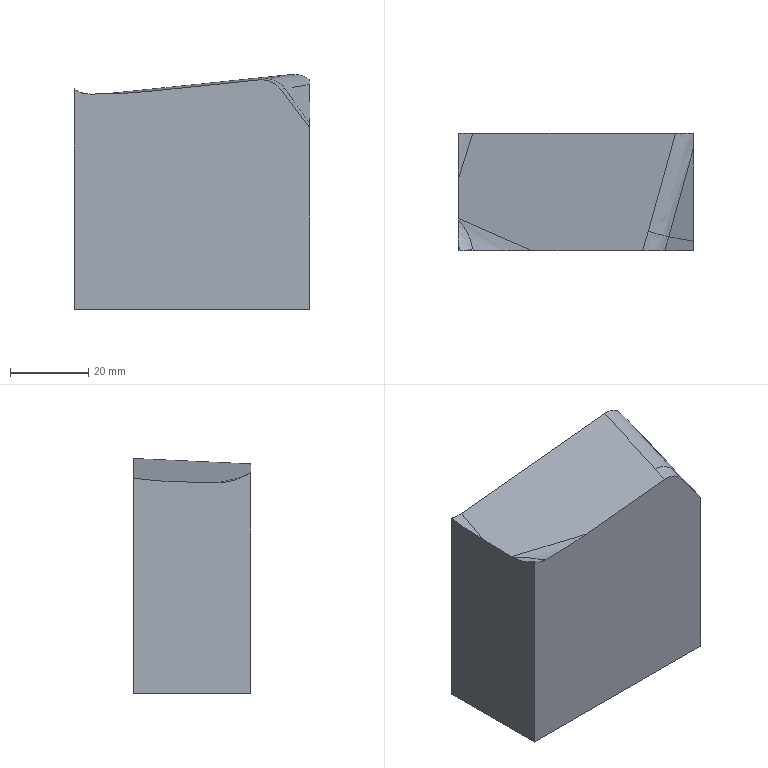Part | NX | features solid 2 | 1 solid | 16 faces | box 60.01 x 30 x 60.012 mm | volume 102012 mm3 | spline 11 | plane 5
STEP:
#1=CARTESIAN_POINT('',(32.377,40.,-15.));
#2=VERTEX_POINT('',#1);
#3=CARTESIAN_POINT('',(32.377,40.,31.446));
#4=VERTEX_POINT('',#3);
#5=CARTESIAN_POINT('',(32.377,40.,-20.));
#6=DIRECTION('',(0.,0.,1.));
#7=VECTOR('',#6,1000.);
#8=LINE('',#5,#7);
#9=EDGE_CURVE('',#2,#4,#8,.T.);
#10=ORIENTED_EDGE('',*,*,#9,.T.);
#11=CARTESIAN_POINT('',(25.028,40.,41.184));
#12=VERTEX_POINT('',#11);
#13=CARTESIAN_POINT('',(32.377,40.,31.446));
#14=CARTESIAN_POINT('',(29.928,40.,34.692));
#15=CARTESIAN_POINT('',(27.478,40.,37.938));
#16=CARTESIAN_POINT('',(25.028,40.,41.184));
#17=B_SPLINE_CURVE_WITH_KNOTS('',3,(#13,#14,#15,#16),.UNSPECIFIED.,.F.,.F.,(4,4),(0.,0.0122),.UNSPECIFIED.);
#18=EDGE_CURVE('',#4,#12,#17,.T.);
#19=ORIENTED_EDGE('',*,*,#18,.T.);
#20=CARTESIAN_POINT('',(19.358,40.,43.587));
#21=VERTEX_POINT('',#20);
#22=CARTESIAN_POINT('',(25.028,40.,41.184));
#23=CARTESIAN_POINT('',(23.722,40.,42.914));
#24=CARTESIAN_POINT('',(21.512,40.,43.811));
#25=CARTESIAN_POINT('',(19.357,40.,43.587));
#26=B_SPLINE_CURVE_WITH_KNOTS('',3,(#22,#23,#24,#25),.UNSPECIFIED.,.F.,.F.,(4,4),(0.,0.006409),.UNSPECIFIED.);
#27=EDGE_CURVE('',#12,#21,#26,.T.);
#28=ORIENTED_EDGE('',*,*,#27,.T.);
#29=CARTESIAN_POINT('',(-8.897,40.,40.647));
#30=VERTEX_POINT('',#29);
#31=CARTESIAN_POINT('',(25.693,40.,44.246));
#32=DIRECTION('',(-0.9946,0.,-0.1035));
#33=VECTOR('',#32,1000.);
#34=LINE('',#31,#33);
#35=EDGE_CURVE('',#30,#21,#34,.F.);
#36=ORIENTED_EDGE('',*,*,#35,.F.);
#37=CARTESIAN_POINT('',(-23.064,40.,39.991));
#38=VERTEX_POINT('',#37);
#39=CARTESIAN_POINT('',(-8.897,40.,40.647));
#40=CARTESIAN_POINT('',(-13.602,40.,40.157));
#41=CARTESIAN_POINT('',(-18.334,40.,39.93));
#42=CARTESIAN_POINT('',(-23.064,40.,39.991));
#43=B_SPLINE_CURVE_WITH_KNOTS('',3,(#39,#40,#41,#42),.UNSPECIFIED.,.F.,.F.,(4,4),(0.,0.01419),.UNSPECIFIED.);
#44=EDGE_CURVE('',#30,#38,#43,.T.);
#45=ORIENTED_EDGE('',*,*,#44,.T.);
#46=CARTESIAN_POINT('',(-23.897,40.,40.002));
#47=VERTEX_POINT('',#46);
#48=CARTESIAN_POINT('',(33.144,40.,39.264));
#49=DIRECTION('',(0.9999,0.,-0.01294));
#50=VECTOR('',#49,1000.);
#51=LINE('',#48,#50);
#52=EDGE_CURVE('',#38,#47,#51,.F.);
#53=ORIENTED_EDGE('',*,*,#52,.T.);
#54=CARTESIAN_POINT('',(-25.828,40.,40.342));
#55=VERTEX_POINT('',#54);
#56=CARTESIAN_POINT('',(-23.897,40.,40.002));
#57=CARTESIAN_POINT('',(-24.555,40.,40.01));
#58=CARTESIAN_POINT('',(-25.207,40.,40.124));
#59=CARTESIAN_POINT('',(-25.828,40.,40.342));
#60=B_SPLINE_CURVE_WITH_KNOTS('',3,(#56,#57,#58,#59),.UNSPECIFIED.,.F.,.F.,(4,4),(0.,0.001968),.UNSPECIFIED.);
#61=EDGE_CURVE('',#47,#55,#60,.T.);
#62=ORIENTED_EDGE('',*,*,#61,.T.);
#63=CARTESIAN_POINT('',(-27.138,40.,40.998));
#64=VERTEX_POINT('',#63);
#65=CARTESIAN_POINT('',(-25.828,40.,40.342));
#66=CARTESIAN_POINT('',(-26.292,40.,40.506));
#67=CARTESIAN_POINT('',(-26.729,40.,40.724));
#68=CARTESIAN_POINT('',(-27.138,40.,40.998));
#69=B_SPLINE_CURVE_WITH_KNOTS('',3,(#65,#66,#67,#68),.UNSPECIFIED.,.F.,.F.,(4,4),(0.,0.001465),.UNSPECIFIED.);
#70=EDGE_CURVE('',#55,#64,#69,.T.);
#71=ORIENTED_EDGE('',*,*,#70,.T.);
#72=CARTESIAN_POINT('',(-27.623,40.,41.321));
#73=VERTEX_POINT('',#72);
#74=CARTESIAN_POINT('',(-27.623,40.,41.321));
#75=CARTESIAN_POINT('',(-27.461,40.,41.214));
#76=CARTESIAN_POINT('',(-27.299,40.,41.106));
#77=CARTESIAN_POINT('',(-27.138,40.,40.998));
#78=B_SPLINE_CURVE_WITH_KNOTS('',3,(#74,#75,#76,#77),.UNSPECIFIED.,.F.,.F.,(4,4),(0.,0.0005827),.UNSPECIFIED.);
#79=EDGE_CURVE('',#73,#64,#78,.T.);
#80=ORIENTED_EDGE('',*,*,#79,.F.);
#81=CARTESIAN_POINT('',(-27.623,40.,-15.));
#82=VERTEX_POINT('',#81);
#83=CARTESIAN_POINT('',(-27.623,40.,-20.));
#84=DIRECTION('',(0.,0.,1.));
#85=VECTOR('',#84,1000.);
#86=LINE('',#83,#85);
#87=EDGE_CURVE('',#82,#73,#86,.T.);
#88=ORIENTED_EDGE('',*,*,#87,.F.);
#89=CARTESIAN_POINT('',(32.377,40.,-15.));
#90=DIRECTION('',(-1.,0.,0.));
#91=VECTOR('',#90,1000.);
#92=LINE('',#89,#91);
#93=EDGE_CURVE('',#2,#82,#92,.T.);
#94=ORIENTED_EDGE('',*,*,#93,.F.);
#95=EDGE_LOOP('',(#10,#19,#28,#36,#45,#53,#62,#71,#80,#88,#94));
#96=FACE_BOUND('',#95,.T.);
#97=CARTESIAN_POINT('',(32.377,40.,-20.));
#98=DIRECTION('',(0.,-1.,0.));
#99=DIRECTION('',(0.,0.,1.));
#100=AXIS2_PLACEMENT_3D('',#97,#98,#99);
#101=PLANE('',#100);
#102=ADVANCED_FACE('',(#96),#101,.T.);
#103=CARTESIAN_POINT('',(27.766,70.,44.978));
#104=VERTEX_POINT('',#103);
#105=CARTESIAN_POINT('',(-23.99,70.,39.593));
#106=VERTEX_POINT('',#105);
#107=CARTESIAN_POINT('',(25.639,70.,44.757));
#108=DIRECTION('',(-0.9946,0.,-0.1035));
#109=VECTOR('',#108,1000.);
#110=LINE('',#107,#109);
#111=EDGE_CURVE('',#104,#106,#110,.T.);
#112=ORIENTED_EDGE('',*,*,#111,.F.);
#113=CARTESIAN_POINT('',(32.377,70.,43.631));
#114=VERTEX_POINT('',#113);
#115=CARTESIAN_POINT('',(27.766,70.,44.978));
#116=CARTESIAN_POINT('',(29.414,70.,45.149));
#117=CARTESIAN_POINT('',(31.089,70.,44.673));
#118=CARTESIAN_POINT('',(32.377,70.,43.631));
#119=B_SPLINE_CURVE_WITH_KNOTS('',3,(#115,#116,#117,#118),.UNSPECIFIED.,.F.,.F.,(4,4),(0.,0.004901),.UNSPECIFIED.);
#120=EDGE_CURVE('',#104,#114,#119,.T.);
#121=ORIENTED_EDGE('',*,*,#120,.T.);
#122=CARTESIAN_POINT('',(32.377,70.,-15.));
#123=VERTEX_POINT('',#122);
#124=CARTESIAN_POINT('',(32.377,70.,-20.));
#125=DIRECTION('',(0.,0.,1.));
#126=VECTOR('',#125,1000.);
#127=LINE('',#124,#126);
#128=EDGE_CURVE('',#123,#114,#127,.T.);
#129=ORIENTED_EDGE('',*,*,#128,.F.);
#130=CARTESIAN_POINT('',(-27.623,70.,-15.));
#131=VERTEX_POINT('',#130);
#132=CARTESIAN_POINT('',(32.377,70.,-15.));
#133=DIRECTION('',(1.,0.,0.));
#134=VECTOR('',#133,1000.);
#135=LINE('',#132,#134);
#136=EDGE_CURVE('',#123,#131,#135,.F.);
#137=ORIENTED_EDGE('',*,*,#136,.T.);
#138=CARTESIAN_POINT('',(-27.623,70.,39.982));
#139=VERTEX_POINT('',#138);
#140=CARTESIAN_POINT('',(-27.623,70.,-20.));
#141=DIRECTION('',(0.,0.,1.));
#142=VECTOR('',#141,1000.);
#143=LINE('',#140,#142);
#144=EDGE_CURVE('',#131,#139,#143,.T.);
#145=ORIENTED_EDGE('',*,*,#144,.T.);
#146=CARTESIAN_POINT('',(-27.623,70.,39.982));
#147=CARTESIAN_POINT('',(-26.447,70.,39.593));
#148=CARTESIAN_POINT('',(-25.221,70.,39.465));
#149=CARTESIAN_POINT('',(-23.99,70.,39.593));
#150=B_SPLINE_CURVE_WITH_KNOTS('',3,(#146,#147,#148,#149),.UNSPECIFIED.,.F.,.F.,(4,4),(0.,0.003655),.UNSPECIFIED.);
#151=EDGE_CURVE('',#139,#106,#150,.T.);
#152=ORIENTED_EDGE('',*,*,#151,.T.);
#153=EDGE_LOOP('',(#112,#121,#129,#137,#145,#152));
#154=FACE_BOUND('',#153,.T.);
#155=CARTESIAN_POINT('',(32.377,70.,-20.));
#156=DIRECTION('',(0.,-1.,0.));
#157=DIRECTION('',(0.,0.,1.));
#158=AXIS2_PLACEMENT_3D('',#155,#156,#157);
#159=PLANE('',#158);
#160=ADVANCED_FACE('',(#154),#159,.F.);
#161=CARTESIAN_POINT('',(32.377,42.373,32.471));
#162=VERTEX_POINT('',#161);
#163=CARTESIAN_POINT('',(32.377,40.,31.446));
#164=CARTESIAN_POINT('',(32.377,40.79,31.789));
#165=CARTESIAN_POINT('',(32.377,41.581,32.131));
#166=CARTESIAN_POINT('',(32.377,42.373,32.471));
#167=B_SPLINE_CURVE_WITH_KNOTS('',3,(#163,#164,#165,#166),.UNSPECIFIED.,.F.,.F.,(4,4),(0.,0.002585),.UNSPECIFIED.);
#168=EDGE_CURVE('',#4,#162,#167,.T.);
#169=ORIENTED_EDGE('',*,*,#168,.F.);
#170=ORIENTED_EDGE('',*,*,#9,.F.);
#171=CARTESIAN_POINT('',(32.377,70.,-15.));
#172=DIRECTION('',(0.,-1.,0.));
#173=VECTOR('',#172,1000.);
#174=LINE('',#171,#173);
#175=EDGE_CURVE('',#123,#2,#174,.T.);
#176=ORIENTED_EDGE('',*,*,#175,.F.);
#177=ORIENTED_EDGE('',*,*,#128,.T.);
#178=CARTESIAN_POINT('',(32.379,66.203,42.403));
#179=VERTEX_POINT('',#178);
#180=CARTESIAN_POINT('',(32.377,66.203,42.405));
#181=CARTESIAN_POINT('',(32.377,67.44,42.904));
#182=CARTESIAN_POINT('',(32.377,68.711,43.294));
#183=CARTESIAN_POINT('',(32.377,70.,43.631));
#184=B_SPLINE_CURVE_WITH_KNOTS('',3,(#180,#181,#182,#183),.UNSPECIFIED.,.F.,.F.,(4,4),(0.00001028,0.004),.UNSPECIFIED.);
#185=EDGE_CURVE('',#179,#114,#184,.T.);
#186=ORIENTED_EDGE('',*,*,#185,.F.);
#187=CARTESIAN_POINT('',(32.377,42.373,32.471));
#188=CARTESIAN_POINT('',(32.377,50.281,35.867));
#189=CARTESIAN_POINT('',(32.377,58.225,39.179));
#190=CARTESIAN_POINT('',(32.377,66.203,42.405));
#191=B_SPLINE_CURVE_WITH_KNOTS('',3,(#187,#188,#189,#190),.UNSPECIFIED.,.F.,.F.,(4,4),(0.,0.02582),.UNSPECIFIED.);
#192=EDGE_CURVE('',#162,#179,#191,.T.);
#193=ORIENTED_EDGE('',*,*,#192,.F.);
#194=EDGE_LOOP('',(#169,#170,#176,#177,#186,#193));
#195=FACE_BOUND('',#194,.T.);
#196=CARTESIAN_POINT('',(32.377,70.,-20.));
#197=DIRECTION('',(-1.,0.,0.));
#198=DIRECTION('',(0.,0.,1.));
#199=AXIS2_PLACEMENT_3D('',#196,#197,#198);
#200=PLANE('',#199);
#201=ADVANCED_FACE('',(#195),#200,.F.);
#202=ORIENTED_EDGE('',*,*,#136,.F.);
#203=ORIENTED_EDGE('',*,*,#175,.T.);
#204=ORIENTED_EDGE('',*,*,#93,.T.);
#205=CARTESIAN_POINT('',(-27.623,70.,-15.));
#206=DIRECTION('',(0.,-1.,0.));
#207=VECTOR('',#206,1000.);
#208=LINE('',#205,#207);
#209=EDGE_CURVE('',#131,#82,#208,.T.);
#210=ORIENTED_EDGE('',*,*,#209,.F.);
#211=EDGE_LOOP('',(#202,#203,#204,#210));
#212=FACE_BOUND('',#211,.T.);
#213=CARTESIAN_POINT('',(32.377,70.,-15.));
#214=DIRECTION('',(0.,0.,-1.));
#215=DIRECTION('',(0.,-1.,0.));
#216=AXIS2_PLACEMENT_3D('',#213,#214,#215);
#217=PLANE('',#216);
#218=ADVANCED_FACE('',(#212),#217,.T.);
#219=CARTESIAN_POINT('',(-27.631,41.344,40.671));
#220=VERTEX_POINT('',#219);
#221=CARTESIAN_POINT('',(-27.623,41.368,40.654));
#222=CARTESIAN_POINT('',(-27.623,40.916,40.886));
#223=CARTESIAN_POINT('',(-27.623,40.46,41.108));
#224=CARTESIAN_POINT('',(-27.623,40.,41.321));
#225=B_SPLINE_CURVE_WITH_KNOTS('',3,(#221,#222,#223,#224),.UNSPECIFIED.,.F.,.F.,(4,4),(0.0005543,0.002076),.UNSPECIFIED.);
#226=EDGE_CURVE('',#220,#73,#225,.T.);
#227=ORIENTED_EDGE('',*,*,#226,.F.);
#228=CARTESIAN_POINT('',(-27.623,47.756,38.836));
#229=VERTEX_POINT('',#228);
#230=CARTESIAN_POINT('',(-27.623,41.327,40.675));
#231=CARTESIAN_POINT('',(-27.623,43.333,39.65));
#232=CARTESIAN_POINT('',(-27.623,45.498,38.84));
#233=CARTESIAN_POINT('',(-27.623,47.755,38.836));
#234=B_SPLINE_CURVE_WITH_KNOTS('',3,(#230,#231,#232,#233),.UNSPECIFIED.,.F.,.F.,(4,4),(0.,0.006751),.UNSPECIFIED.);
#235=EDGE_CURVE('',#220,#229,#234,.T.);
#236=ORIENTED_EDGE('',*,*,#235,.T.);
#237=CARTESIAN_POINT('',(-27.623,48.203,38.84));
#238=VERTEX_POINT('',#237);
#239=CARTESIAN_POINT('',(-27.623,47.757,38.836));
#240=CARTESIAN_POINT('',(-27.623,47.905,38.836));
#241=CARTESIAN_POINT('',(-27.623,48.054,38.837));
#242=CARTESIAN_POINT('',(-27.623,48.203,38.84));
#243=B_SPLINE_CURVE_WITH_KNOTS('',3,(#239,#240,#241,#242),.UNSPECIFIED.,.F.,.F.,(4,4),(0.005811,0.006257),.UNSPECIFIED.);
#244=EDGE_CURVE('',#229,#238,#243,.T.);
#245=ORIENTED_EDGE('',*,*,#244,.T.);
#246=CARTESIAN_POINT('',(-27.623,58.443,39.016));
#247=VERTEX_POINT('',#246);
#248=CARTESIAN_POINT('',(-27.623,68.981,39.197));
#249=DIRECTION('',(0.,0.9999,0.01721));
#250=VECTOR('',#249,1000.);
#251=LINE('',#248,#250);
#252=EDGE_CURVE('',#247,#238,#251,.F.);
#253=ORIENTED_EDGE('',*,*,#252,.F.);
#254=CARTESIAN_POINT('',(-27.623,58.443,39.016));
#255=CARTESIAN_POINT('',(-27.623,62.313,39.082));
#256=CARTESIAN_POINT('',(-27.623,66.175,39.393));
#257=CARTESIAN_POINT('',(-27.623,70.,39.982));
#258=B_SPLINE_CURVE_WITH_KNOTS('',3,(#254,#255,#256,#257),.UNSPECIFIED.,.F.,.F.,(4,4),(0.,0.0116),.UNSPECIFIED.);
#259=EDGE_CURVE('',#247,#139,#258,.T.);
#260=ORIENTED_EDGE('',*,*,#259,.T.);
#261=ORIENTED_EDGE('',*,*,#144,.F.);
#262=ORIENTED_EDGE('',*,*,#209,.T.);
#263=ORIENTED_EDGE('',*,*,#87,.T.);
#264=EDGE_LOOP('',(#227,#236,#245,#253,#260,#261,#262,#263));
#265=FACE_BOUND('',#264,.T.);
#266=CARTESIAN_POINT('',(-27.623,70.,-20.));
#267=DIRECTION('',(-1.,0.,0.));
#268=DIRECTION('',(0.,0.,1.));
#269=AXIS2_PLACEMENT_3D('',#266,#267,#268);
#270=PLANE('',#269);
#271=ADVANCED_FACE('',(#265),#270,.T.);
#272=ORIENTED_EDGE('',*,*,#192,.T.);
#273=CARTESIAN_POINT('',(26.058,43.542,41.352));
#274=VERTEX_POINT('',#273);
#275=CARTESIAN_POINT('',(26.058,43.542,41.352));
#276=CARTESIAN_POINT('',(28.23,51.078,41.709));
#277=CARTESIAN_POINT('',(30.337,58.632,42.058));
#278=CARTESIAN_POINT('',(32.38,66.203,42.402));
#279=B_SPLINE_CURVE_WITH_KNOTS('',3,(#275,#276,#277,#278),.UNSPECIFIED.,.F.,.F.,(4,4),(0.,0.215),.UNSPECIFIED.);
#280=EDGE_CURVE('',#274,#179,#279,.T.);
#281=ORIENTED_EDGE('',*,*,#280,.F.);
#282=CARTESIAN_POINT('',(32.377,42.373,32.471));
#283=CARTESIAN_POINT('',(30.271,42.763,35.431));
#284=CARTESIAN_POINT('',(28.165,43.153,38.392));
#285=CARTESIAN_POINT('',(26.058,43.542,41.352));
#286=B_SPLINE_CURVE_WITH_KNOTS('',3,(#282,#283,#284,#285),.UNSPECIFIED.,.F.,.F.,(4,4),(0.2573,1.),.UNSPECIFIED.);
#287=EDGE_CURVE('',#274,#162,#286,.F.);
#288=ORIENTED_EDGE('',*,*,#287,.T.);
#289=EDGE_LOOP('',(#272,#281,#288));
#290=FACE_BOUND('',#289,.T.);
#291=CARTESIAN_POINT('',(26.02,43.549,41.406));
#292=CARTESIAN_POINT('',(32.415,42.366,32.417));
#293=CARTESIAN_POINT('',(27.276,48.108,41.699));
#294=CARTESIAN_POINT('',(33.673,46.933,32.711));
#295=CARTESIAN_POINT('',(28.514,52.671,41.985));
#296=CARTESIAN_POINT('',(34.914,51.505,32.998));
#297=CARTESIAN_POINT('',(29.737,57.239,42.265));
#298=CARTESIAN_POINT('',(36.139,56.082,33.279));
#299=CARTESIAN_POINT('',(30.943,61.812,42.539));
#300=CARTESIAN_POINT('',(37.347,60.663,33.553));
#301=CARTESIAN_POINT('',(32.133,66.39,42.806));
#302=CARTESIAN_POINT('',(38.539,65.249,33.82));
#303=B_SPLINE_SURFACE_WITH_KNOTS('',5,1,((#291,#292),(#293,#294),(#295,#296),(#297,#298),(#299,#300),(#301,#302)),.RULED_SURF.,.F.,.F.,.F.,(6,6),(2,2),(0.,0.2163),(0.002694,0.5483),.PIECEWISE_BEZIER_KNOTS.);
#304=ADVANCED_FACE('',(#290),#303,.F.);
#305=ORIENTED_EDGE('',*,*,#259,.F.);
#306=CARTESIAN_POINT('',(-27.623,58.443,39.016));
#307=CARTESIAN_POINT('',(-26.412,62.295,39.208));
#308=CARTESIAN_POINT('',(-25.201,66.148,39.4));
#309=CARTESIAN_POINT('',(-23.99,70.,39.593));
#310=B_SPLINE_CURVE_WITH_KNOTS('',3,(#306,#307,#308,#309),.UNSPECIFIED.,.F.,.F.,(4,4),(0.0582,0.1357),.UNSPECIFIED.);
#311=EDGE_CURVE('',#106,#247,#310,.F.);
#312=ORIENTED_EDGE('',*,*,#311,.F.);
#313=ORIENTED_EDGE('',*,*,#151,.F.);
#314=EDGE_LOOP('',(#305,#312,#313));
#315=FACE_BOUND('',#314,.T.);
#316=CARTESIAN_POINT('',(-30.976,59.398,39.459));
#317=CARTESIAN_POINT('',(-27.3,71.094,40.043));
#318=CARTESIAN_POINT('',(-29.897,59.08,39.05));
#319=CARTESIAN_POINT('',(-26.221,70.775,39.634));
#320=CARTESIAN_POINT('',(-28.768,58.732,38.902));
#321=CARTESIAN_POINT('',(-25.092,70.428,39.485));
#322=CARTESIAN_POINT('',(-27.644,58.374,39.012));
#323=CARTESIAN_POINT('',(-23.969,70.069,39.596));
#324=(BOUNDED_SURFACE()B_SPLINE_SURFACE(3,1,((#316,#317),(#318,#319),(#320,#321),(#322,#323)),.CYLINDRICAL_SURF.,.F.,.F.,.F.)B_SPLINE_SURFACE_WITH_KNOTS((4,4),(2,2),(0.3966,1.),(0.0648,0.1426),.PIECEWISE_BEZIER_KNOTS.)GEOMETRIC_REPRESENTATION_ITEM()RATIONAL_B_SPLINE_SURFACE(((0.9683,0.9683),(0.9627,0.9627),(0.9733,0.9733),(1.,1.)))REPRESENTATION_ITEM('')SURFACE());
#325=ADVANCED_FACE('',(#315),#324,.T.);
#326=ORIENTED_EDGE('',*,*,#79,.T.);
#327=CARTESIAN_POINT('',(-27.63,41.345,40.671));
#328=CARTESIAN_POINT('',(-27.409,40.899,40.761));
#329=CARTESIAN_POINT('',(-27.246,40.45,40.868));
#330=CARTESIAN_POINT('',(-27.138,40.,40.998));
#331=B_SPLINE_CURVE_WITH_KNOTS('',3,(#327,#328,#329,#330),.UNSPECIFIED.,.F.,.F.,(4,4),(0.7229,0.9658),.UNSPECIFIED.);
#332=EDGE_CURVE('',#64,#220,#331,.F.);
#333=ORIENTED_EDGE('',*,*,#332,.T.);
#334=ORIENTED_EDGE('',*,*,#226,.T.);
#335=EDGE_LOOP('',(#326,#333,#334));
#336=FACE_BOUND('',#335,.T.);
#337=CARTESIAN_POINT('',(-27.454,39.756,41.32));
#338=CARTESIAN_POINT('',(-26.789,40.247,40.653));
#339=CARTESIAN_POINT('',(-27.726,40.139,41.33));
#340=CARTESIAN_POINT('',(-27.06,40.629,40.663));
#341=CARTESIAN_POINT('',(-28.004,40.516,41.329));
#342=CARTESIAN_POINT('',(-27.338,41.006,40.662));
#343=CARTESIAN_POINT('',(-28.29,40.887,41.317));
#344=CARTESIAN_POINT('',(-27.624,41.377,40.65));
#345=(BOUNDED_SURFACE()B_SPLINE_SURFACE(3,1,((#337,#338),(#339,#340),(#341,#342),(#343,#344)),.CYLINDRICAL_SURF.,.F.,.F.,.F.)B_SPLINE_SURFACE_WITH_KNOTS((4,4),(2,2),(0.5041,0.5582),(0.9085,0.9756),.PIECEWISE_BEZIER_KNOTS.)GEOMETRIC_REPRESENTATION_ITEM()RATIONAL_B_SPLINE_SURFACE(((0.9243,0.9243),(0.9243,0.9243),(0.9247,0.9247),(0.9253,0.9253)))REPRESENTATION_ITEM('')SURFACE());
#346=ADVANCED_FACE('',(#336),#345,.F.);
#347=CARTESIAN_POINT('',(-24.011,40.415,39.9));
#348=VERTEX_POINT('',#347);
#349=CARTESIAN_POINT('',(-25.828,40.,40.342));
#350=CARTESIAN_POINT('',(-25.245,40.108,40.099));
#351=CARTESIAN_POINT('',(-24.628,40.249,39.949));
#352=CARTESIAN_POINT('',(-24.011,40.415,39.9));
#353=B_SPLINE_CURVE_WITH_KNOTS('',3,(#349,#350,#351,#352),.UNSPECIFIED.,.F.,.F.,(4,4),(0.433,1.),.UNSPECIFIED.);
#354=EDGE_CURVE('',#55,#348,#353,.T.);
#355=ORIENTED_EDGE('',*,*,#354,.T.);
#356=CARTESIAN_POINT('',(-24.011,40.415,39.9));
#357=CARTESIAN_POINT('',(-24.162,41.791,39.558));
#358=CARTESIAN_POINT('',(-25.008,44.578,39.117));
#359=CARTESIAN_POINT('',(-26.684,46.808,38.928));
#360=CARTESIAN_POINT('',(-27.623,47.756,38.836));
#361=B_SPLINE_CURVE_WITH_KNOTS('',3,(#356,#357,#358,#359,#360),.UNSPECIFIED.,.F.,.F.,(4,1,4),(0.,0.4318,0.8635),.UNSPECIFIED.);
#362=EDGE_CURVE('',#229,#348,#361,.F.);
#363=ORIENTED_EDGE('',*,*,#362,.F.);
#364=ORIENTED_EDGE('',*,*,#235,.F.);
#365=ORIENTED_EDGE('',*,*,#332,.F.);
#366=ORIENTED_EDGE('',*,*,#70,.F.);
#367=EDGE_LOOP('',(#355,#363,#364,#365,#366));
#368=FACE_BOUND('',#367,.T.);
#369=CARTESIAN_POINT('',(-27.095,39.81,41.054));
#370=CARTESIAN_POINT('',(-26.548,39.87,40.657));
#371=CARTESIAN_POINT('',(-25.95,39.963,40.335));
#372=CARTESIAN_POINT('',(-25.317,40.087,40.097));
#373=CARTESIAN_POINT('',(-24.664,40.239,39.952));
#374=CARTESIAN_POINT('',(-24.011,40.415,39.9));
#375=CARTESIAN_POINT('',(-27.265,40.637,40.804));
#376=CARTESIAN_POINT('',(-26.714,40.787,40.377));
#377=CARTESIAN_POINT('',(-26.111,40.975,40.031));
#378=CARTESIAN_POINT('',(-25.47,41.197,39.778));
#379=CARTESIAN_POINT('',(-24.811,41.447,39.626));
#380=CARTESIAN_POINT('',(-24.154,41.717,39.576));
#381=CARTESIAN_POINT('',(-27.595,41.479,40.615));
#382=CARTESIAN_POINT('',(-27.048,41.716,40.158));
#383=CARTESIAN_POINT('',(-26.445,41.999,39.79));
#384=CARTESIAN_POINT('',(-25.803,42.321,39.526));
#385=CARTESIAN_POINT('',(-25.143,42.671,39.376));
#386=CARTESIAN_POINT('',(-24.487,43.038,39.338));
#387=CARTESIAN_POINT('',(-28.093,42.286,40.488));
#388=CARTESIAN_POINT('',(-27.557,42.603,39.999));
#389=CARTESIAN_POINT('',(-26.961,42.976,39.611));
#390=CARTESIAN_POINT('',(-26.325,43.392,39.339));
#391=CARTESIAN_POINT('',(-25.672,43.839,39.195));
#392=CARTESIAN_POINT('',(-25.025,44.298,39.18));
#393=CARTESIAN_POINT('',(-28.873,43.227,40.371));
#394=CARTESIAN_POINT('',(-28.356,43.632,39.843));
#395=CARTESIAN_POINT('',(-27.777,44.105,39.427));
#396=CARTESIAN_POINT('',(-27.156,44.632,39.147));
#397=CARTESIAN_POINT('',(-26.52,45.19,39.014));
#398=CARTESIAN_POINT('',(-25.894,45.757,39.027));
#399=CARTESIAN_POINT('',(-29.788,44.054,40.293));
#400=CARTESIAN_POINT('',(-29.296,44.528,39.725));
#401=CARTESIAN_POINT('',(-28.74,45.087,39.282));
#402=CARTESIAN_POINT('',(-28.143,45.709,38.992));
#403=CARTESIAN_POINT('',(-27.534,46.364,38.867));
#404=CARTESIAN_POINT('',(-26.938,47.023,38.906));
#405=CARTESIAN_POINT('',(-29.991,44.227,40.277));
#406=CARTESIAN_POINT('',(-29.505,44.716,39.7));
#407=CARTESIAN_POINT('',(-28.955,45.293,39.252));
#408=CARTESIAN_POINT('',(-28.363,45.934,38.96));
#409=CARTESIAN_POINT('',(-27.76,46.61,38.837));
#410=CARTESIAN_POINT('',(-27.171,47.288,38.881));
#411=CARTESIAN_POINT('',(-30.2,44.395,40.262));
#412=CARTESIAN_POINT('',(-29.719,44.898,39.678));
#413=CARTESIAN_POINT('',(-29.175,45.491,39.224));
#414=CARTESIAN_POINT('',(-28.589,46.152,38.929));
#415=CARTESIAN_POINT('',(-27.992,46.847,38.807));
#416=CARTESIAN_POINT('',(-27.411,47.543,38.857));
#417=CARTESIAN_POINT('',(-30.413,44.558,40.249));
#418=CARTESIAN_POINT('',(-29.938,45.073,39.656));
#419=CARTESIAN_POINT('',(-29.4,45.682,39.196));
#420=CARTESIAN_POINT('',(-28.821,46.361,38.898));
#421=CARTESIAN_POINT('',(-28.23,47.075,38.778));
#422=CARTESIAN_POINT('',(-27.657,47.79,38.833));
#423=B_SPLINE_SURFACE_WITH_KNOTS('',5,5,((#369,#370,#371,#372,#373,#374),(#375,#376,#377,#378,#379,#380),(#381,#382,#383,#384,#385,#386),(#387,#388,#389,#390,#391,#392),(#393,#394,#395,#396,#397,#398),(#399,#400,#401,#402,#403,#404),(#405,#406,#407,#408,#409,#410),(#411,#412,#413,#414,#415,#416),(#417,#418,#419,#420,#421,#422)),.UNSPECIFIED.,.F.,.F.,.F.,(6,3,6),(6,6),(0.,0.6808,0.8687),(0.,1.),.UNSPECIFIED.);
#424=ADVANCED_FACE('',(#368),#423,.F.);
#425=CARTESIAN_POINT('',(20.799,44.941,43.822));
#426=VERTEX_POINT('',#425);
#427=CARTESIAN_POINT('',(27.766,70.,44.978));
#428=CARTESIAN_POINT('',(25.524,61.629,44.6));
#429=CARTESIAN_POINT('',(23.203,53.282,44.215));
#430=CARTESIAN_POINT('',(20.799,44.941,43.822));
#431=B_SPLINE_CURVE_WITH_KNOTS('',3,(#427,#428,#429,#430),.UNSPECIFIED.,.F.,.F.,(4,4),(0.7615,1.),.UNSPECIFIED.);
#432=EDGE_CURVE('',#426,#104,#431,.F.);
#433=ORIENTED_EDGE('',*,*,#432,.F.);
#434=CARTESIAN_POINT('',(20.799,44.941,43.822));
#435=CARTESIAN_POINT('',(21.995,44.591,43.94));
#436=CARTESIAN_POINT('',(23.224,44.247,43.734));
#437=CARTESIAN_POINT('',(24.378,43.94,43.192));
#438=CARTESIAN_POINT('',(25.344,43.7,42.367));
#439=CARTESIAN_POINT('',(26.058,43.542,41.352));
#440=B_SPLINE_CURVE_WITH_KNOTS('',5,(#434,#435,#436,#437,#438,#439),.UNSPECIFIED.,.F.,.F.,(6,6),(0.,1.),.PIECEWISE_BEZIER_KNOTS.);
#441=EDGE_CURVE('',#426,#274,#440,.T.);
#442=ORIENTED_EDGE('',*,*,#441,.T.);
#443=ORIENTED_EDGE('',*,*,#280,.T.);
#444=ORIENTED_EDGE('',*,*,#185,.T.);
#445=ORIENTED_EDGE('',*,*,#120,.F.);
#446=EDGE_LOOP('',(#433,#442,#443,#444,#445));
#447=FACE_BOUND('',#446,.T.);
#448=CARTESIAN_POINT('',(20.799,44.941,43.822));
#449=CARTESIAN_POINT('',(21.995,44.591,43.94));
#450=CARTESIAN_POINT('',(23.224,44.247,43.734));
#451=CARTESIAN_POINT('',(24.378,43.94,43.192));
#452=CARTESIAN_POINT('',(25.344,43.7,42.367));
#453=CARTESIAN_POINT('',(26.058,43.542,41.352));
#454=CARTESIAN_POINT('',(21.555,47.565,43.946));
#455=CARTESIAN_POINT('',(22.751,47.217,44.064));
#456=CARTESIAN_POINT('',(23.981,46.875,43.858));
#457=CARTESIAN_POINT('',(25.136,46.57,43.316));
#458=CARTESIAN_POINT('',(26.103,46.332,42.492));
#459=CARTESIAN_POINT('',(26.817,46.175,41.477));
#460=CARTESIAN_POINT('',(22.303,50.183,44.068));
#461=CARTESIAN_POINT('',(23.5,49.837,44.187));
#462=CARTESIAN_POINT('',(24.73,49.498,43.981));
#463=CARTESIAN_POINT('',(25.885,49.195,43.44));
#464=CARTESIAN_POINT('',(26.852,48.959,42.615));
#465=CARTESIAN_POINT('',(27.567,48.803,41.6));
#466=CARTESIAN_POINT('',(23.046,52.811,44.191));
#467=CARTESIAN_POINT('',(24.244,52.468,44.31));
#468=CARTESIAN_POINT('',(25.474,52.131,44.104));
#469=CARTESIAN_POINT('',(26.63,51.83,43.563));
#470=CARTESIAN_POINT('',(27.598,51.596,42.738));
#471=CARTESIAN_POINT('',(28.313,51.441,41.723));
#472=CARTESIAN_POINT('',(24.517,58.061,44.434));
#473=CARTESIAN_POINT('',(25.716,57.723,44.553));
#474=CARTESIAN_POINT('',(26.948,57.391,44.348));
#475=CARTESIAN_POINT('',(28.105,57.095,43.807));
#476=CARTESIAN_POINT('',(29.074,56.864,42.983));
#477=CARTESIAN_POINT('',(29.79,56.712,41.968));
#478=CARTESIAN_POINT('',(25.963,63.321,44.675));
#479=CARTESIAN_POINT('',(27.163,62.988,44.794));
#480=CARTESIAN_POINT('',(28.396,62.66,44.589));
#481=CARTESIAN_POINT('',(29.554,62.368,44.048));
#482=CARTESIAN_POINT('',(30.524,62.141,43.224));
#483=CARTESIAN_POINT('',(31.241,61.991,42.21));
#484=CARTESIAN_POINT('',(26.679,65.951,44.795));
#485=CARTESIAN_POINT('',(27.879,65.62,44.914));
#486=CARTESIAN_POINT('',(29.113,65.295,44.709));
#487=CARTESIAN_POINT('',(30.272,65.005,44.168));
#488=CARTESIAN_POINT('',(31.242,64.779,43.345));
#489=CARTESIAN_POINT('',(31.959,64.631,42.331));
#490=CARTESIAN_POINT('',(27.39,68.589,44.914));
#491=CARTESIAN_POINT('',(28.591,68.261,45.034));
#492=CARTESIAN_POINT('',(29.825,67.938,44.829));
#493=CARTESIAN_POINT('',(30.985,67.65,44.288));
#494=CARTESIAN_POINT('',(31.955,67.427,43.465));
#495=CARTESIAN_POINT('',(32.673,67.279,42.451));
#496=CARTESIAN_POINT('',(28.094,71.229,45.033));
#497=CARTESIAN_POINT('',(29.296,70.903,45.153));
#498=CARTESIAN_POINT('',(30.531,70.583,44.948));
#499=CARTESIAN_POINT('',(31.691,70.297,44.407));
#500=CARTESIAN_POINT('',(32.662,70.075,43.584));
#501=CARTESIAN_POINT('',(33.38,69.929,42.57));
#502=CARTESIAN_POINT('',(28.096,71.235,45.033));
#503=CARTESIAN_POINT('',(29.297,70.909,45.153));
#504=CARTESIAN_POINT('',(30.533,70.589,44.948));
#505=CARTESIAN_POINT('',(31.693,70.304,44.408));
#506=CARTESIAN_POINT('',(32.664,70.082,43.584));
#507=CARTESIAN_POINT('',(33.381,69.936,42.57));
#508=CARTESIAN_POINT('',(28.097,71.241,45.034));
#509=CARTESIAN_POINT('',(29.299,70.915,45.153));
#510=CARTESIAN_POINT('',(30.534,70.595,44.948));
#511=CARTESIAN_POINT('',(31.694,70.31,44.408));
#512=CARTESIAN_POINT('',(32.665,70.088,43.584));
#513=CARTESIAN_POINT('',(33.383,69.942,42.57));
#514=CARTESIAN_POINT('',(28.099,71.248,45.034));
#515=CARTESIAN_POINT('',(29.301,70.922,45.153));
#516=CARTESIAN_POINT('',(30.536,70.601,44.949));
#517=CARTESIAN_POINT('',(31.696,70.316,44.408));
#518=CARTESIAN_POINT('',(32.667,70.094,43.585));
#519=CARTESIAN_POINT('',(33.385,69.948,42.571));
#520=B_SPLINE_SURFACE_WITH_KNOTS('',5,5,((#448,#449,#450,#451,#452,#453),(#454,#455,#456,#457,#458,#459),(#460,#461,#462,#463,#464,#465),(#466,#467,#468,#469,#470,#471),(#472,#473,#474,#475,#476,#477),(#478,#479,#480,#481,#482,#483),(#484,#485,#486,#487,#488,#489),(#490,#491,#492,#493,#494,#495),(#496,#497,#498,#499,#500,#501),(#502,#503,#504,#505,#506,#507),(#508,#509,#510,#511,#512,#513),(#514,#515,#516,#517,#518,#519)),.UNSPECIFIED.,.F.,.F.,.F.,(6,3,3,6),(6,6),(0.,0.125,0.25,0.2503),(0.,1.),.UNSPECIFIED.);
#521=ADVANCED_FACE('',(#447),#520,.F.);
#522=ORIENTED_EDGE('',*,*,#35,.T.);
#523=CARTESIAN_POINT('',(19.358,40.,43.587));
#524=CARTESIAN_POINT('',(19.879,41.77,43.671));
#525=CARTESIAN_POINT('',(20.36,43.417,43.75));
#526=CARTESIAN_POINT('',(20.799,44.941,43.822));
#527=B_SPLINE_CURVE_WITH_KNOTS('',3,(#523,#524,#525,#526),.UNSPECIFIED.,.F.,.F.,(4,4),(0.6466,1.),.UNSPECIFIED.);
#528=EDGE_CURVE('',#21,#426,#527,.T.);
#529=ORIENTED_EDGE('',*,*,#528,.T.);
#530=ORIENTED_EDGE('',*,*,#432,.T.);
#531=ORIENTED_EDGE('',*,*,#111,.T.);
#532=ORIENTED_EDGE('',*,*,#311,.T.);
#533=ORIENTED_EDGE('',*,*,#252,.T.);
#534=CARTESIAN_POINT('',(-27.623,48.203,38.84));
#535=CARTESIAN_POINT('',(-21.381,45.469,39.442));
#536=CARTESIAN_POINT('',(-15.139,42.734,40.044));
#537=CARTESIAN_POINT('',(-8.897,40.,40.647));
#538=B_SPLINE_CURVE_WITH_KNOTS('',3,(#534,#535,#536,#537),.UNSPECIFIED.,.F.,.F.,(4,4),(0.0206,0.4402),.UNSPECIFIED.);
#539=EDGE_CURVE('',#30,#238,#538,.F.);
#540=ORIENTED_EDGE('',*,*,#539,.F.);
#541=EDGE_LOOP('',(#522,#529,#530,#531,#532,#533,#540));
#542=FACE_BOUND('',#541,.T.);
#543=CARTESIAN_POINT('',(-27.989,39.889,38.658));
#544=CARTESIAN_POINT('',(-27.933,70.383,39.189));
#545=CARTESIAN_POINT('',(28.043,39.685,44.485));
#546=CARTESIAN_POINT('',(28.098,70.18,45.016));
#547=B_SPLINE_SURFACE_WITH_KNOTS('',1,1,((#543,#544),(#545,#546)),.PLANE_SURF.,.F.,.F.,.F.,(2,2),(2,2),(0.03315,0.6741),(0.06737,0.2429),.PIECEWISE_BEZIER_KNOTS.);
#548=ADVANCED_FACE('',(#542),#547,.T.);
#549=CARTESIAN_POINT('',(-23.897,40.,40.002));
#550=CARTESIAN_POINT('',(-23.933,40.138,39.968));
#551=CARTESIAN_POINT('',(-23.971,40.277,39.934));
#552=CARTESIAN_POINT('',(-24.011,40.415,39.9));
#553=B_SPLINE_CURVE_WITH_KNOTS('',3,(#549,#550,#551,#552),.UNSPECIFIED.,.F.,.F.,(4,4),(0.9799,1.),.UNSPECIFIED.);
#554=EDGE_CURVE('',#47,#348,#553,.T.);
#555=ORIENTED_EDGE('',*,*,#554,.T.);
#556=ORIENTED_EDGE('',*,*,#354,.F.);
#557=ORIENTED_EDGE('',*,*,#61,.F.);
#558=EDGE_LOOP('',(#555,#556,#557));
#559=FACE_BOUND('',#558,.T.);
#560=CARTESIAN_POINT('',(-25.754,39.62,40.446));
#561=CARTESIAN_POINT('',(-25.396,39.677,40.298));
#562=CARTESIAN_POINT('',(-25.029,39.744,40.179));
#563=CARTESIAN_POINT('',(-24.654,39.82,40.089));
#564=CARTESIAN_POINT('',(-24.275,39.905,40.03));
#565=CARTESIAN_POINT('',(-23.896,39.997,40.002));
#566=CARTESIAN_POINT('',(-25.77,39.696,40.426));
#567=CARTESIAN_POINT('',(-25.413,39.755,40.279));
#568=CARTESIAN_POINT('',(-25.047,39.823,40.159));
#569=CARTESIAN_POINT('',(-24.673,39.901,40.069));
#570=CARTESIAN_POINT('',(-24.296,39.987,40.01));
#571=CARTESIAN_POINT('',(-23.918,40.081,39.982));
#572=CARTESIAN_POINT('',(-25.786,39.772,40.406));
#573=CARTESIAN_POINT('',(-25.431,39.832,40.259));
#574=CARTESIAN_POINT('',(-25.065,39.902,40.139));
#575=CARTESIAN_POINT('',(-24.693,39.981,40.049));
#576=CARTESIAN_POINT('',(-24.317,40.069,39.99));
#577=CARTESIAN_POINT('',(-23.94,40.165,39.961));
#578=CARTESIAN_POINT('',(-25.803,39.847,40.386));
#579=CARTESIAN_POINT('',(-25.449,39.909,40.239));
#580=CARTESIAN_POINT('',(-25.085,39.981,40.119));
#581=CARTESIAN_POINT('',(-24.713,40.062,40.029));
#582=CARTESIAN_POINT('',(-24.339,40.151,39.97));
#583=CARTESIAN_POINT('',(-23.963,40.248,39.941));
#584=CARTESIAN_POINT('',(-25.821,39.923,40.366));
#585=CARTESIAN_POINT('',(-25.468,39.986,40.219));
#586=CARTESIAN_POINT('',(-25.104,40.059,40.1));
#587=CARTESIAN_POINT('',(-24.734,40.142,40.01));
#588=CARTESIAN_POINT('',(-24.361,40.233,39.95));
#589=CARTESIAN_POINT('',(-23.987,40.331,39.92));
#590=CARTESIAN_POINT('',(-25.839,39.998,40.347));
#591=CARTESIAN_POINT('',(-25.487,40.063,40.199));
#592=CARTESIAN_POINT('',(-25.125,40.138,40.08));
#593=CARTESIAN_POINT('',(-24.756,40.222,39.99));
#594=CARTESIAN_POINT('',(-24.383,40.315,39.93));
#595=CARTESIAN_POINT('',(-24.011,40.415,39.9));
#596=B_SPLINE_SURFACE_WITH_KNOTS('',5,5,((#560,#561,#562,#563,#564,#565),(#566,#567,#568,#569,#570,#571),(#572,#573,#574,#575,#576,#577),(#578,#579,#580,#581,#582,#583),(#584,#585,#586,#587,#588,#589),(#590,#591,#592,#593,#594,#595)),.UNSPECIFIED.,.F.,.F.,.F.,(6,6),(6,6),(0.9798,1.),(0.4296,1.),.PIECEWISE_BEZIER_KNOTS.);
#597=ADVANCED_FACE('',(#559),#596,.F.);
#598=ORIENTED_EDGE('',*,*,#539,.T.);
#599=ORIENTED_EDGE('',*,*,#244,.F.);
#600=ORIENTED_EDGE('',*,*,#362,.T.);
#601=CARTESIAN_POINT('',(-24.011,40.415,39.9));
#602=CARTESIAN_POINT('',(-23.695,40.277,39.93));
#603=CARTESIAN_POINT('',(-23.379,40.138,39.961));
#604=CARTESIAN_POINT('',(-23.064,40.,39.991));
#605=B_SPLINE_CURVE_WITH_KNOTS('',3,(#601,#602,#603,#604),.UNSPECIFIED.,.F.,.F.,(4,4),(0.,0.02494),.UNSPECIFIED.);
#606=EDGE_CURVE('',#348,#38,#605,.T.);
#607=ORIENTED_EDGE('',*,*,#606,.T.);
#608=ORIENTED_EDGE('',*,*,#44,.F.);
#609=EDGE_LOOP('',(#598,#599,#600,#607,#608));
#610=FACE_BOUND('',#609,.T.);
#611=CARTESIAN_POINT('',(-27.735,48.252,38.829));
#612=CARTESIAN_POINT('',(-8.785,39.951,40.658));
#613=CARTESIAN_POINT('',(-28.493,46.497,38.72));
#614=CARTESIAN_POINT('',(-9.543,38.196,40.548));
#615=CARTESIAN_POINT('',(-29.272,44.756,38.883));
#616=CARTESIAN_POINT('',(-10.322,36.454,40.712));
#617=CARTESIAN_POINT('',(-30.056,43.063,39.316));
#618=CARTESIAN_POINT('',(-11.106,34.761,41.145));
#619=(BOUNDED_SURFACE()B_SPLINE_SURFACE(3,1,((#611,#612),(#613,#614),(#615,#616),(#617,#618)),.CYLINDRICAL_SURF.,.F.,.F.,.F.)B_SPLINE_SURFACE_WITH_KNOTS((4,4),(2,2),(0.,1.),(0.02368,0.4406),.PIECEWISE_BEZIER_KNOTS.)GEOMETRIC_REPRESENTATION_ITEM()RATIONAL_B_SPLINE_SURFACE(((1.,1.),(0.9932,0.9932),(0.9932,0.9932),(1.,1.)))REPRESENTATION_ITEM('')SURFACE());
#620=ADVANCED_FACE('',(#610),#619,.T.);
#621=CARTESIAN_POINT('',(25.028,40.,41.184));
#622=CARTESIAN_POINT('',(25.384,41.213,41.242));
#623=CARTESIAN_POINT('',(25.729,42.398,41.298));
#624=CARTESIAN_POINT('',(26.058,43.542,41.352));
#625=B_SPLINE_CURVE_WITH_KNOTS('',3,(#621,#622,#623,#624),.UNSPECIFIED.,.F.,.F.,(4,4),(0.7637,1.),.UNSPECIFIED.);
#626=EDGE_CURVE('',#12,#274,#625,.T.);
#627=ORIENTED_EDGE('',*,*,#626,.T.);
#628=ORIENTED_EDGE('',*,*,#441,.F.);
#629=ORIENTED_EDGE('',*,*,#528,.F.);
#630=ORIENTED_EDGE('',*,*,#27,.F.);
#631=EDGE_LOOP('',(#627,#628,#629,#630));
#632=FACE_BOUND('',#631,.T.);
#633=CARTESIAN_POINT('',(19.348,39.969,43.585));
#634=CARTESIAN_POINT('',(20.541,39.612,43.703));
#635=CARTESIAN_POINT('',(21.768,39.26,43.497));
#636=CARTESIAN_POINT('',(22.921,38.946,42.954));
#637=CARTESIAN_POINT('',(23.885,38.701,42.129));
#638=CARTESIAN_POINT('',(24.599,38.539,41.114));
#639=CARTESIAN_POINT('',(19.652,40.999,43.634));
#640=CARTESIAN_POINT('',(20.846,40.643,43.753));
#641=CARTESIAN_POINT('',(22.073,40.292,43.546));
#642=CARTESIAN_POINT('',(23.225,39.98,43.004));
#643=CARTESIAN_POINT('',(24.19,39.736,42.179));
#644=CARTESIAN_POINT('',(24.904,39.574,41.164));
#645=CARTESIAN_POINT('',(19.95,42.014,43.683));
#646=CARTESIAN_POINT('',(21.144,41.659,43.801));
#647=CARTESIAN_POINT('',(22.372,41.31,43.595));
#648=CARTESIAN_POINT('',(23.524,40.998,43.053));
#649=CARTESIAN_POINT('',(24.49,40.755,42.227));
#650=CARTESIAN_POINT('',(25.203,40.595,41.212));
#651=CARTESIAN_POINT('',(20.241,43.012,43.73));
#652=CARTESIAN_POINT('',(21.436,42.658,43.849));
#653=CARTESIAN_POINT('',(22.664,42.31,43.642));
#654=CARTESIAN_POINT('',(23.817,42.,43.1));
#655=CARTESIAN_POINT('',(24.783,41.758,42.275));
#656=CARTESIAN_POINT('',(25.496,41.598,41.26));
#657=CARTESIAN_POINT('',(20.525,43.989,43.777));
#658=CARTESIAN_POINT('',(21.72,43.637,43.895));
#659=CARTESIAN_POINT('',(22.948,43.291,43.689));
#660=CARTESIAN_POINT('',(24.102,42.982,43.147));
#661=CARTESIAN_POINT('',(25.068,42.741,42.322));
#662=CARTESIAN_POINT('',(25.782,42.582,41.307));
#663=CARTESIAN_POINT('',(20.799,44.941,43.822));
#664=CARTESIAN_POINT('',(21.995,44.591,43.94));
#665=CARTESIAN_POINT('',(23.224,44.247,43.734));
#666=CARTESIAN_POINT('',(24.378,43.94,43.192));
#667=CARTESIAN_POINT('',(25.344,43.7,42.367));
#668=CARTESIAN_POINT('',(26.058,43.542,41.352));
#669=B_SPLINE_SURFACE_WITH_KNOTS('',5,5,((#633,#634,#635,#636,#637,#638),(#639,#640,#641,#642,#643,#644),(#645,#646,#647,#648,#649,#650),(#651,#652,#653,#654,#655,#656),(#657,#658,#659,#660,#661,#662),(#663,#664,#665,#666,#667,#668)),.UNSPECIFIED.,.F.,.F.,.F.,(6,6),(6,6),(0.6696,1.),(0.,1.),.PIECEWISE_BEZIER_KNOTS.);
#670=ADVANCED_FACE('',(#632),#669,.F.);
#671=ORIENTED_EDGE('',*,*,#606,.F.);
#672=ORIENTED_EDGE('',*,*,#554,.F.);
#673=ORIENTED_EDGE('',*,*,#52,.F.);
#674=EDGE_LOOP('',(#671,#672,#673));
#675=FACE_BOUND('',#674,.T.);
#676=CARTESIAN_POINT('',(-24.016,39.998,40.004));
#677=CARTESIAN_POINT('',(-23.058,39.995,39.992));
#678=CARTESIAN_POINT('',(-24.016,40.417,39.899));
#679=CARTESIAN_POINT('',(-23.058,40.414,39.887));
#680=B_SPLINE_SURFACE_WITH_KNOTS('',1,1,((#676,#677),(#678,#679)),.PLANE_SURF.,.F.,.F.,.F.,(2,2),(2,2),(0.9837,0.9941),(0.4313,0.4455),.PIECEWISE_BEZIER_KNOTS.);
#681=ADVANCED_FACE('',(#675),#680,.F.);
#682=ORIENTED_EDGE('',*,*,#168,.T.);
#683=ORIENTED_EDGE('',*,*,#287,.F.);
#684=ORIENTED_EDGE('',*,*,#626,.F.);
#685=ORIENTED_EDGE('',*,*,#18,.F.);
#686=EDGE_LOOP('',(#682,#683,#684,#685));
#687=FACE_BOUND('',#686,.T.);
#688=CARTESIAN_POINT('',(31.991,38.61,31.354));
#689=CARTESIAN_POINT('',(32.393,39.885,31.376));
#690=CARTESIAN_POINT('',(32.757,41.099,31.42));
#691=CARTESIAN_POINT('',(33.078,42.244,31.486));
#692=CARTESIAN_POINT('',(30.583,38.887,33.339));
#693=CARTESIAN_POINT('',(30.982,40.157,33.364));
#694=CARTESIAN_POINT('',(31.344,41.366,33.409));
#695=CARTESIAN_POINT('',(31.663,42.505,33.475));
#696=CARTESIAN_POINT('',(29.175,39.163,35.325));
#697=CARTESIAN_POINT('',(29.571,40.429,35.352));
#698=CARTESIAN_POINT('',(29.93,41.632,35.398));
#699=CARTESIAN_POINT('',(30.248,42.767,35.463));
#700=CARTESIAN_POINT('',(27.767,39.439,37.31));
#701=CARTESIAN_POINT('',(28.16,40.7,37.34));
#702=CARTESIAN_POINT('',(28.517,41.899,37.386));
#703=CARTESIAN_POINT('',(28.834,43.029,37.452));
#704=CARTESIAN_POINT('',(26.36,39.715,39.296));
#705=CARTESIAN_POINT('',(26.749,40.971,39.328));
#706=CARTESIAN_POINT('',(27.103,42.166,39.375));
#707=CARTESIAN_POINT('',(27.419,43.29,39.44));
#708=CARTESIAN_POINT('',(24.952,39.991,41.281));
#709=CARTESIAN_POINT('',(25.338,41.243,41.315));
#710=CARTESIAN_POINT('',(25.69,42.432,41.364));
#711=CARTESIAN_POINT('',(26.004,43.552,41.428));
#712=B_SPLINE_SURFACE_WITH_KNOTS('',5,3,((#688,#689,#690,#691),(#692,#693,#694,#695),(#696,#697,#698,#699),(#700,#701,#702,#703),(#704,#705,#706,#707),(#708,#709,#710,#711)),.UNSPECIFIED.,.F.,.F.,.F.,(6,6),(4,4),(0.242,0.9075),(0.8544,1.),.PIECEWISE_BEZIER_KNOTS.);
#713=ADVANCED_FACE('',(#687),#712,.F.);
#714=CLOSED_SHELL('',(#102,#160,#201,#218,#271,#304,#325,#346,#424,#521,#548,#597,#620,#670,#681,#713));
#715=MANIFOLD_SOLID_BREP('',#714);
#716=(LENGTH_UNIT()NAMED_UNIT(*)SI_UNIT(.MILLI.,.METRE.));
#717=UNCERTAINTY_MEASURE_WITH_UNIT(LENGTH_MEASURE(0.112),#716,'','');
#718=(NAMED_UNIT(*)PLANE_ANGLE_UNIT()SI_UNIT($,.RADIAN.));
#719=(NAMED_UNIT(*)SI_UNIT($,.STERADIAN.)SOLID_ANGLE_UNIT());
#720=(GEOMETRIC_REPRESENTATION_CONTEXT(3)GLOBAL_UNCERTAINTY_ASSIGNED_CONTEXT((#717))GLOBAL_UNIT_ASSIGNED_CONTEXT((#716,#718,#719))REPRESENTATION_CONTEXT('',''));
#721=ADVANCED_BREP_SHAPE_REPRESENTATION('',(#715),#720);